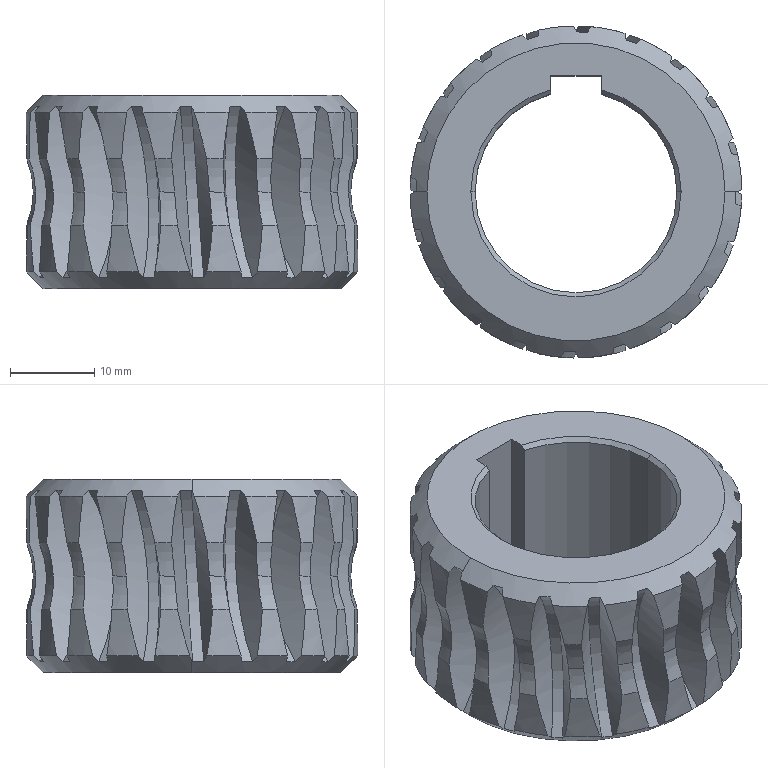Part | SolidWorks | features Chamfer 2, CirPattern 1, Helix 1, ICE 1, Revolution 1, SweepCut 1 | 1 solid | 158 faces | box 39.446 x 39.446 x 23 mm | volume 13124 mm3 | spline 60 | cylinder 43 | torus 40 | cone 10 | plane 5 | commonest cylinder face diameters 39.45 x40 24 x3